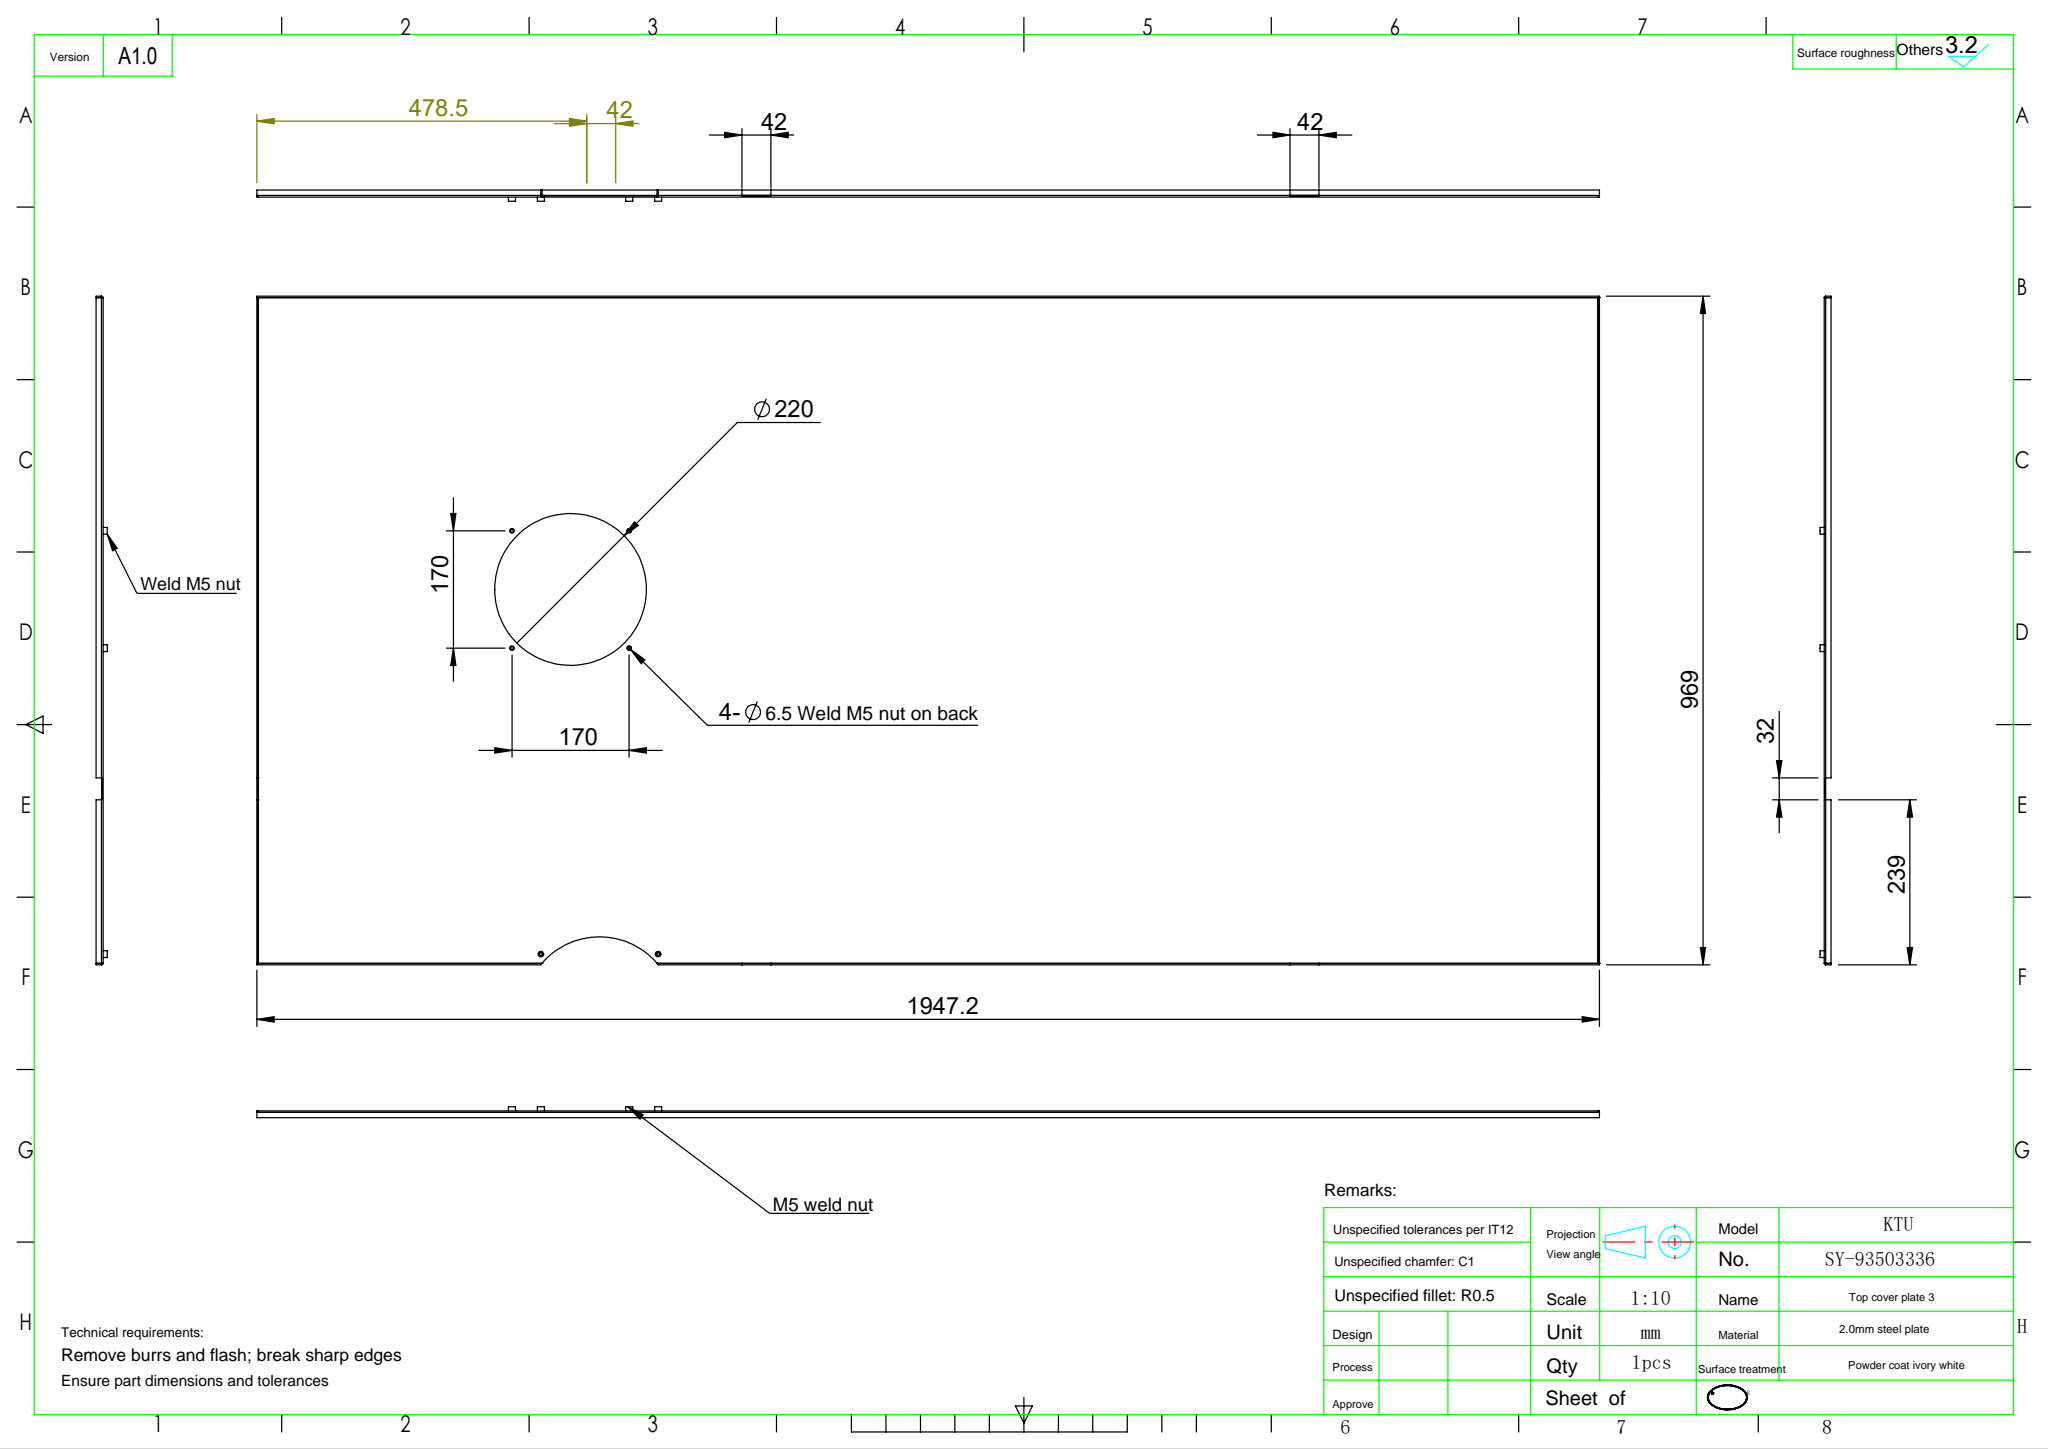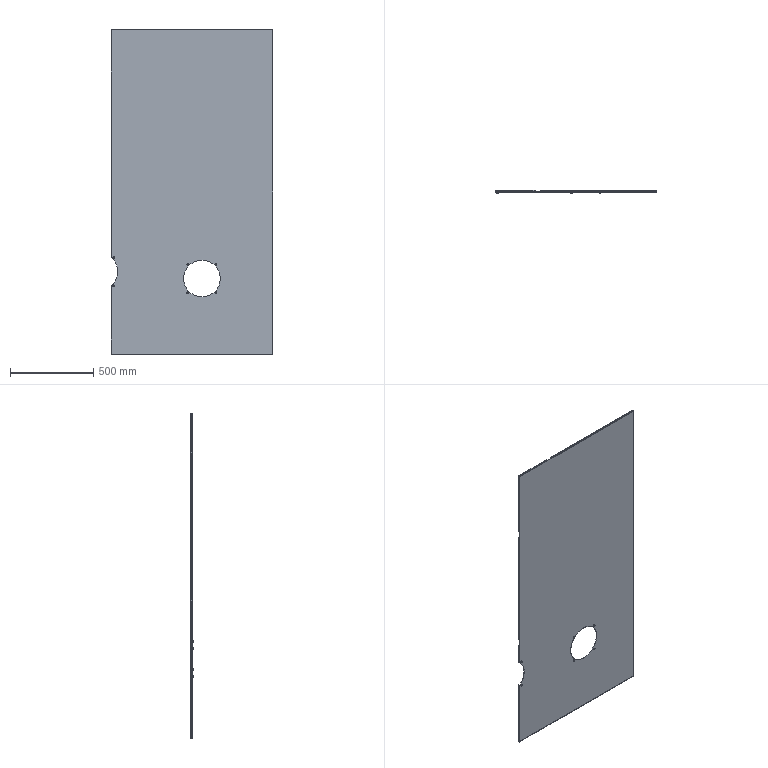Part | SolidWorks | features ICE 5, Cut 3, EdgeFlange 1, FlatPattern 1, HoleWzd 1, MirrorPattern 1, SMBaseFlange 1, SheetMetal 1 | 5 solids | 130 faces | box 969 x 16 x 1947 mm | volume 3772126 mm3 | plane 81 | cylinder 49 | commonest cylinder face diameters 4.2 x12 10 x12 6.5 x8 0.4 x5 4.4 x5 8 x4